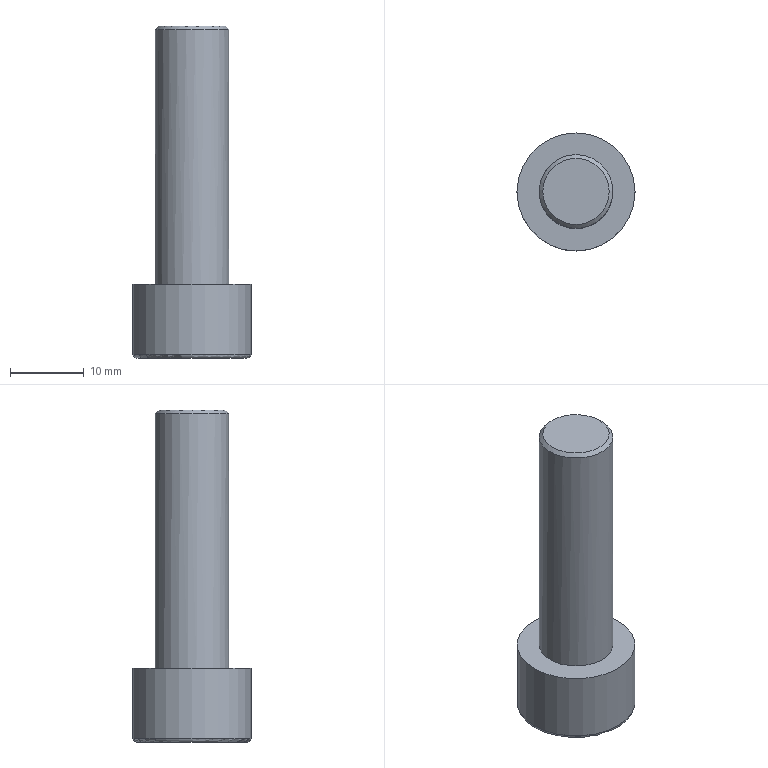Part | NX | features 模具.stp<1>[90] 2 | 1 solid | 14 faces | box 16 x 16 x 45 mm | volume 4476 mm3 | plane 10 | cylinder 2 | cone 1 | torus 1 | commonest cylinder face diameters 10 x1 16 x1
STEP:
#1=CARTESIAN_POINT('',(-57.5,-206.881,-239.5));
#2=VERTEX_POINT('',#1);
#3=CARTESIAN_POINT('',(-53.5,-209.191,-239.5));
#4=VERTEX_POINT('',#3);
#5=CARTESIAN_POINT('',(-57.5,-206.881,-239.5));
#6=DIRECTION('',(0.866,-0.5,0.));
#7=VECTOR('',#6,1000.);
#8=LINE('',#5,#7);
#9=EDGE_CURVE('',#2,#4,#8,.T.);
#10=ORIENTED_EDGE('',*,*,#9,.T.);
#11=CARTESIAN_POINT('',(-53.5,-213.809,-239.5));
#12=VERTEX_POINT('',#11);
#13=CARTESIAN_POINT('',(-53.5,-209.191,-239.5));
#14=DIRECTION('',(0.,-1.,0.));
#15=VECTOR('',#14,1000.);
#16=LINE('',#13,#15);
#17=EDGE_CURVE('',#4,#12,#16,.T.);
#18=ORIENTED_EDGE('',*,*,#17,.T.);
#19=CARTESIAN_POINT('',(-57.5,-216.119,-239.5));
#20=VERTEX_POINT('',#19);
#21=CARTESIAN_POINT('',(-53.5,-213.809,-239.5));
#22=DIRECTION('',(-0.866,-0.5,0.));
#23=VECTOR('',#22,1000.);
#24=LINE('',#21,#23);
#25=EDGE_CURVE('',#12,#20,#24,.T.);
#26=ORIENTED_EDGE('',*,*,#25,.T.);
#27=CARTESIAN_POINT('',(-61.5,-213.809,-239.5));
#28=VERTEX_POINT('',#27);
#29=CARTESIAN_POINT('',(-57.5,-216.119,-239.5));
#30=DIRECTION('',(-0.866,0.5,0.));
#31=VECTOR('',#30,1000.);
#32=LINE('',#29,#31);
#33=EDGE_CURVE('',#20,#28,#32,.T.);
#34=ORIENTED_EDGE('',*,*,#33,.T.);
#35=CARTESIAN_POINT('',(-61.5,-209.191,-239.5));
#36=VERTEX_POINT('',#35);
#37=CARTESIAN_POINT('',(-61.5,-213.809,-239.5));
#38=DIRECTION('',(0.,1.,0.));
#39=VECTOR('',#38,1000.);
#40=LINE('',#37,#39);
#41=EDGE_CURVE('',#28,#36,#40,.T.);
#42=ORIENTED_EDGE('',*,*,#41,.T.);
#43=CARTESIAN_POINT('',(-61.5,-209.191,-239.5));
#44=DIRECTION('',(0.866,0.5,0.));
#45=VECTOR('',#44,1000.);
#46=LINE('',#43,#45);
#47=EDGE_CURVE('',#36,#2,#46,.T.);
#48=ORIENTED_EDGE('',*,*,#47,.T.);
#49=EDGE_LOOP('',(#10,#18,#26,#34,#42,#48));
#50=FACE_BOUND('',#49,.T.);
#51=CARTESIAN_POINT('',(-57.5,-211.5,-239.5));
#52=DIRECTION('',(0.,0.,1.));
#53=DIRECTION('',(1.,0.,0.));
#54=AXIS2_PLACEMENT_3D('',#51,#52,#53);
#55=PLANE('',#54);
#56=ADVANCED_FACE('',(#50),#55,.F.);
#57=CARTESIAN_POINT('',(-57.5,-206.881,-244.5));
#58=VERTEX_POINT('',#57);
#59=CARTESIAN_POINT('',(-53.5,-209.191,-244.5));
#60=VERTEX_POINT('',#59);
#61=CARTESIAN_POINT('',(-57.5,-206.881,-244.5));
#62=DIRECTION('',(0.866,-0.5,0.));
#63=VECTOR('',#62,1000.);
#64=LINE('',#61,#63);
#65=EDGE_CURVE('',#58,#60,#64,.T.);
#66=ORIENTED_EDGE('',*,*,#65,.T.);
#67=CARTESIAN_POINT('',(-53.5,-209.191,-239.5));
#68=DIRECTION('',(0.,0.,-1.));
#69=VECTOR('',#68,1000.);
#70=LINE('',#67,#69);
#71=EDGE_CURVE('',#4,#60,#70,.T.);
#72=ORIENTED_EDGE('',*,*,#71,.F.);
#73=ORIENTED_EDGE('',*,*,#9,.F.);
#74=CARTESIAN_POINT('',(-57.5,-206.881,-239.5));
#75=DIRECTION('',(0.,0.,-1.));
#76=VECTOR('',#75,1000.);
#77=LINE('',#74,#76);
#78=EDGE_CURVE('',#2,#58,#77,.T.);
#79=ORIENTED_EDGE('',*,*,#78,.T.);
#80=EDGE_LOOP('',(#66,#72,#73,#79));
#81=FACE_BOUND('',#80,.T.);
#82=CARTESIAN_POINT('',(-55.5,-208.036,-242.));
#83=DIRECTION('',(0.5,0.866,0.));
#84=DIRECTION('',(0.,0.,-1.));
#85=AXIS2_PLACEMENT_3D('',#82,#83,#84);
#86=PLANE('',#85);
#87=ADVANCED_FACE('',(#81),#86,.F.);
#88=CARTESIAN_POINT('',(-53.5,-213.809,-244.5));
#89=VERTEX_POINT('',#88);
#90=CARTESIAN_POINT('',(-53.5,-209.191,-244.5));
#91=DIRECTION('',(0.,-1.,0.));
#92=VECTOR('',#91,1000.);
#93=LINE('',#90,#92);
#94=EDGE_CURVE('',#60,#89,#93,.T.);
#95=ORIENTED_EDGE('',*,*,#94,.T.);
#96=CARTESIAN_POINT('',(-53.5,-213.809,-239.5));
#97=DIRECTION('',(0.,0.,-1.));
#98=VECTOR('',#97,1000.);
#99=LINE('',#96,#98);
#100=EDGE_CURVE('',#12,#89,#99,.T.);
#101=ORIENTED_EDGE('',*,*,#100,.F.);
#102=ORIENTED_EDGE('',*,*,#17,.F.);
#103=ORIENTED_EDGE('',*,*,#71,.T.);
#104=EDGE_LOOP('',(#95,#101,#102,#103));
#105=FACE_BOUND('',#104,.T.);
#106=CARTESIAN_POINT('',(-53.5,-211.5,-242.));
#107=DIRECTION('',(1.,0.,0.));
#108=DIRECTION('',(0.,0.,-1.));
#109=AXIS2_PLACEMENT_3D('',#106,#107,#108);
#110=PLANE('',#109);
#111=ADVANCED_FACE('',(#105),#110,.F.);
#112=CARTESIAN_POINT('',(-57.5,-216.119,-244.5));
#113=VERTEX_POINT('',#112);
#114=CARTESIAN_POINT('',(-53.5,-213.809,-244.5));
#115=DIRECTION('',(-0.866,-0.5,0.));
#116=VECTOR('',#115,1000.);
#117=LINE('',#114,#116);
#118=EDGE_CURVE('',#89,#113,#117,.T.);
#119=ORIENTED_EDGE('',*,*,#118,.T.);
#120=CARTESIAN_POINT('',(-57.5,-216.119,-239.5));
#121=DIRECTION('',(0.,0.,-1.));
#122=VECTOR('',#121,1000.);
#123=LINE('',#120,#122);
#124=EDGE_CURVE('',#20,#113,#123,.T.);
#125=ORIENTED_EDGE('',*,*,#124,.F.);
#126=ORIENTED_EDGE('',*,*,#25,.F.);
#127=ORIENTED_EDGE('',*,*,#100,.T.);
#128=EDGE_LOOP('',(#119,#125,#126,#127));
#129=FACE_BOUND('',#128,.T.);
#130=CARTESIAN_POINT('',(-55.5,-214.964,-242.));
#131=DIRECTION('',(0.5,-0.866,0.));
#132=DIRECTION('',(0.,0.,-1.));
#133=AXIS2_PLACEMENT_3D('',#130,#131,#132);
#134=PLANE('',#133);
#135=ADVANCED_FACE('',(#129),#134,.F.);
#136=CARTESIAN_POINT('',(-61.5,-213.809,-244.5));
#137=VERTEX_POINT('',#136);
#138=CARTESIAN_POINT('',(-57.5,-216.119,-244.5));
#139=DIRECTION('',(-0.866,0.5,0.));
#140=VECTOR('',#139,1000.);
#141=LINE('',#138,#140);
#142=EDGE_CURVE('',#113,#137,#141,.T.);
#143=ORIENTED_EDGE('',*,*,#142,.T.);
#144=CARTESIAN_POINT('',(-61.5,-213.809,-239.5));
#145=DIRECTION('',(0.,0.,-1.));
#146=VECTOR('',#145,1000.);
#147=LINE('',#144,#146);
#148=EDGE_CURVE('',#28,#137,#147,.T.);
#149=ORIENTED_EDGE('',*,*,#148,.F.);
#150=ORIENTED_EDGE('',*,*,#33,.F.);
#151=ORIENTED_EDGE('',*,*,#124,.T.);
#152=EDGE_LOOP('',(#143,#149,#150,#151));
#153=FACE_BOUND('',#152,.T.);
#154=CARTESIAN_POINT('',(-59.5,-214.964,-242.));
#155=DIRECTION('',(-0.5,-0.866,0.));
#156=DIRECTION('',(-0.866,0.5,0.));
#157=AXIS2_PLACEMENT_3D('',#154,#155,#156);
#158=PLANE('',#157);
#159=ADVANCED_FACE('',(#153),#158,.F.);
#160=CARTESIAN_POINT('',(-61.5,-209.191,-244.5));
#161=VERTEX_POINT('',#160);
#162=CARTESIAN_POINT('',(-61.5,-213.809,-244.5));
#163=DIRECTION('',(0.,1.,0.));
#164=VECTOR('',#163,1000.);
#165=LINE('',#162,#164);
#166=EDGE_CURVE('',#137,#161,#165,.T.);
#167=ORIENTED_EDGE('',*,*,#166,.T.);
#168=CARTESIAN_POINT('',(-61.5,-209.191,-239.5));
#169=DIRECTION('',(0.,0.,-1.));
#170=VECTOR('',#169,1000.);
#171=LINE('',#168,#170);
#172=EDGE_CURVE('',#36,#161,#171,.T.);
#173=ORIENTED_EDGE('',*,*,#172,.F.);
#174=ORIENTED_EDGE('',*,*,#41,.F.);
#175=ORIENTED_EDGE('',*,*,#148,.T.);
#176=EDGE_LOOP('',(#167,#173,#174,#175));
#177=FACE_BOUND('',#176,.T.);
#178=CARTESIAN_POINT('',(-61.5,-211.5,-242.));
#179=DIRECTION('',(-1.,0.,0.));
#180=DIRECTION('',(0.,0.,1.));
#181=AXIS2_PLACEMENT_3D('',#178,#179,#180);
#182=PLANE('',#181);
#183=ADVANCED_FACE('',(#177),#182,.F.);
#184=CARTESIAN_POINT('',(-61.5,-209.191,-244.5));
#185=DIRECTION('',(0.866,0.5,0.));
#186=VECTOR('',#185,1000.);
#187=LINE('',#184,#186);
#188=EDGE_CURVE('',#161,#58,#187,.T.);
#189=ORIENTED_EDGE('',*,*,#188,.T.);
#190=ORIENTED_EDGE('',*,*,#78,.F.);
#191=ORIENTED_EDGE('',*,*,#47,.F.);
#192=ORIENTED_EDGE('',*,*,#172,.T.);
#193=EDGE_LOOP('',(#189,#190,#191,#192));
#194=FACE_BOUND('',#193,.T.);
#195=CARTESIAN_POINT('',(-59.5,-208.036,-242.));
#196=DIRECTION('',(-0.5,0.866,0.));
#197=DIRECTION('',(0.,0.,1.));
#198=AXIS2_PLACEMENT_3D('',#195,#196,#197);
#199=PLANE('',#198);
#200=ADVANCED_FACE('',(#194),#199,.F.);
#201=CARTESIAN_POINT('',(-52.5,-211.5,-200.));
#202=VERTEX_POINT('',#201);
#203=CARTESIAN_POINT('',(-57.5,-211.5,-200.));
#204=DIRECTION('',(0.,0.,-1.));
#205=DIRECTION('',(1.,0.,0.));
#206=AXIS2_PLACEMENT_3D('',#203,#204,#205);
#207=CIRCLE('',#206,5.);
#208=EDGE_CURVE('',#202,#202,#207,.T.);
#209=ORIENTED_EDGE('',*,*,#208,.F.);
#210=EDGE_LOOP('',(#209));
#211=FACE_BOUND('',#210,.T.);
#212=CARTESIAN_POINT('',(-53.,-211.5,-199.5));
#213=VERTEX_POINT('',#212);
#214=CARTESIAN_POINT('',(-57.5,-211.5,-199.5));
#215=DIRECTION('',(0.,0.,1.));
#216=DIRECTION('',(1.,0.,0.));
#217=AXIS2_PLACEMENT_3D('',#214,#215,#216);
#218=CIRCLE('',#217,4.5);
#219=EDGE_CURVE('',#213,#213,#218,.T.);
#220=ORIENTED_EDGE('',*,*,#219,.F.);
#221=EDGE_LOOP('',(#220));
#222=FACE_BOUND('',#221,.T.);
#223=CARTESIAN_POINT('',(-57.5,-211.5,-200.));
#224=DIRECTION('',(0.,0.,-1.));
#225=DIRECTION('',(-1.,0.,0.));
#226=AXIS2_PLACEMENT_3D('',#223,#224,#225);
#227=CONICAL_SURFACE('',#226,5.,0.7854);
#228=ADVANCED_FACE('',(#211,#222),#227,.T.);
#229=CARTESIAN_POINT('',(-57.5,-206.5,-234.5));
#230=VERTEX_POINT('',#229);
#231=CARTESIAN_POINT('',(-57.5,-211.5,-234.5));
#232=DIRECTION('',(0.,0.,1.));
#233=DIRECTION('',(0.,1.,0.));
#234=AXIS2_PLACEMENT_3D('',#231,#232,#233);
#235=CIRCLE('',#234,5.);
#236=EDGE_CURVE('',#230,#230,#235,.T.);
#237=ORIENTED_EDGE('',*,*,#236,.T.);
#238=EDGE_LOOP('',(#237));
#239=FACE_BOUND('',#238,.T.);
#240=ORIENTED_EDGE('',*,*,#208,.T.);
#241=EDGE_LOOP('',(#240));
#242=FACE_BOUND('',#241,.T.);
#243=CARTESIAN_POINT('',(-57.5,-211.5,-199.5));
#244=DIRECTION('',(0.,0.,-1.));
#245=DIRECTION('',(0.,1.,0.));
#246=AXIS2_PLACEMENT_3D('',#243,#244,#245);
#247=CYLINDRICAL_SURFACE('',#246,5.);
#248=ADVANCED_FACE('',(#239,#242),#247,.T.);
#249=ORIENTED_EDGE('',*,*,#219,.T.);
#250=EDGE_LOOP('',(#249));
#251=FACE_BOUND('',#250,.T.);
#252=CARTESIAN_POINT('',(-57.5,-211.5,-199.5));
#253=DIRECTION('',(0.,0.,1.));
#254=DIRECTION('',(1.,0.,0.));
#255=AXIS2_PLACEMENT_3D('',#252,#253,#254);
#256=PLANE('',#255);
#257=ADVANCED_FACE('',(#251),#256,.T.);
#258=CARTESIAN_POINT('',(-65.5,-211.5,-244.));
#259=VERTEX_POINT('',#258);
#260=CARTESIAN_POINT('',(-57.5,-211.5,-244.));
#261=DIRECTION('',(0.,0.,1.));
#262=DIRECTION('',(-1.,0.,0.));
#263=AXIS2_PLACEMENT_3D('',#260,#261,#262);
#264=CIRCLE('',#263,8.);
#265=EDGE_CURVE('',#259,#259,#264,.T.);
#266=ORIENTED_EDGE('',*,*,#265,.F.);
#267=EDGE_LOOP('',(#266));
#268=FACE_BOUND('',#267,.T.);
#269=CARTESIAN_POINT('',(-65.,-211.5,-244.5));
#270=VERTEX_POINT('',#269);
#271=CARTESIAN_POINT('',(-57.5,-211.5,-244.5));
#272=DIRECTION('',(0.,0.,-1.));
#273=DIRECTION('',(-1.,0.,0.));
#274=AXIS2_PLACEMENT_3D('',#271,#272,#273);
#275=CIRCLE('',#274,7.5);
#276=EDGE_CURVE('',#270,#270,#275,.T.);
#277=ORIENTED_EDGE('',*,*,#276,.F.);
#278=EDGE_LOOP('',(#277));
#279=FACE_BOUND('',#278,.T.);
#280=CARTESIAN_POINT('',(-57.5,-211.5,-244.));
#281=DIRECTION('',(0.,0.,-1.));
#282=DIRECTION('',(-1.,0.,0.));
#283=AXIS2_PLACEMENT_3D('',#280,#281,#282);
#284=TOROIDAL_SURFACE('',#283,7.5,0.5);
#285=ADVANCED_FACE('',(#268,#279),#284,.T.);
#286=CARTESIAN_POINT('',(-57.5,-203.5,-234.5));
#287=VERTEX_POINT('',#286);
#288=CARTESIAN_POINT('',(-57.5,-211.5,-234.5));
#289=DIRECTION('',(0.,0.,-1.));
#290=DIRECTION('',(0.,1.,0.));
#291=AXIS2_PLACEMENT_3D('',#288,#289,#290);
#292=CIRCLE('',#291,8.);
#293=EDGE_CURVE('',#287,#287,#292,.T.);
#294=ORIENTED_EDGE('',*,*,#293,.T.);
#295=EDGE_LOOP('',(#294));
#296=FACE_BOUND('',#295,.T.);
#297=ORIENTED_EDGE('',*,*,#265,.T.);
#298=EDGE_LOOP('',(#297));
#299=FACE_BOUND('',#298,.T.);
#300=CARTESIAN_POINT('',(-57.5,-211.5,-234.5));
#301=DIRECTION('',(0.,0.,-1.));
#302=DIRECTION('',(0.,1.,0.));
#303=AXIS2_PLACEMENT_3D('',#300,#301,#302);
#304=CYLINDRICAL_SURFACE('',#303,8.);
#305=ADVANCED_FACE('',(#296,#299),#304,.T.);
#306=ORIENTED_EDGE('',*,*,#293,.F.);
#307=EDGE_LOOP('',(#306));
#308=FACE_BOUND('',#307,.T.);
#309=ORIENTED_EDGE('',*,*,#236,.F.);
#310=EDGE_LOOP('',(#309));
#311=FACE_BOUND('',#310,.T.);
#312=CARTESIAN_POINT('',(-57.5,-211.5,-234.5));
#313=DIRECTION('',(0.,0.,1.));
#314=DIRECTION('',(1.,0.,0.));
#315=AXIS2_PLACEMENT_3D('',#312,#313,#314);
#316=PLANE('',#315);
#317=ADVANCED_FACE('',(#308,#311),#316,.T.);
#318=ORIENTED_EDGE('',*,*,#276,.T.);
#319=EDGE_LOOP('',(#318));
#320=FACE_BOUND('',#319,.T.);
#321=ORIENTED_EDGE('',*,*,#188,.F.);
#322=ORIENTED_EDGE('',*,*,#166,.F.);
#323=ORIENTED_EDGE('',*,*,#142,.F.);
#324=ORIENTED_EDGE('',*,*,#118,.F.);
#325=ORIENTED_EDGE('',*,*,#94,.F.);
#326=ORIENTED_EDGE('',*,*,#65,.F.);
#327=EDGE_LOOP('',(#321,#322,#323,#324,#325,#326));
#328=FACE_BOUND('',#327,.T.);
#329=CARTESIAN_POINT('',(-57.5,-211.5,-244.5));
#330=DIRECTION('',(0.,0.,-1.));
#331=DIRECTION('',(0.,-1.,0.));
#332=AXIS2_PLACEMENT_3D('',#329,#330,#331);
#333=PLANE('',#332);
#334=ADVANCED_FACE('',(#320,#328),#333,.T.);
#335=CLOSED_SHELL('',(#56,#87,#111,#135,#159,#183,#200,#228,#248,#257,#285,#305,#317,#334));
#336=MANIFOLD_SOLID_BREP('',#335);
#337=(LENGTH_UNIT()NAMED_UNIT(*)SI_UNIT(.MILLI.,.METRE.));
#338=UNCERTAINTY_MEASURE_WITH_UNIT(LENGTH_MEASURE(0.00001),#337,'','');
#339=(NAMED_UNIT(*)PLANE_ANGLE_UNIT()SI_UNIT($,.RADIAN.));
#340=(NAMED_UNIT(*)SI_UNIT($,.STERADIAN.)SOLID_ANGLE_UNIT());
#341=(GEOMETRIC_REPRESENTATION_CONTEXT(3)GLOBAL_UNCERTAINTY_ASSIGNED_CONTEXT((#338))GLOBAL_UNIT_ASSIGNED_CONTEXT((#337,#339,#340))REPRESENTATION_CONTEXT('',''));
#342=ADVANCED_BREP_SHAPE_REPRESENTATION('',(#336),#341);